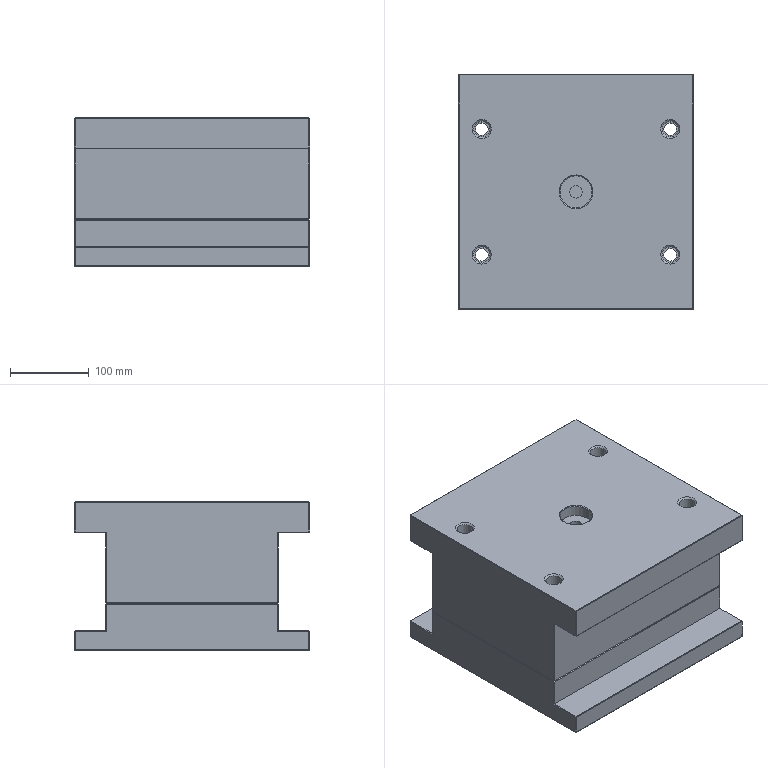NC program | NX | posted with a generic post | part box 300 x 300 x 190 mm
Lines 6041 to 6235 of 6235:
(刀补 , TOOL : D10JING)
N12062 T09 M6
N12064 G54
N12066 G17 G0 G90 X-120. Y80. S3500 M3
N12068 G43 Z30. H9
N12070 Z0.5
N12072 G41 G94 G1 X-120.011 Y79.901 F1200. D9
N12074 G3 X-117.05 Y80. R1.482
N12076 X-117.05 Y80. Z-2. I-2.95 J0.
N12078 X-117.05 Y80. Z-4.5 I-2.95 J0.
N12080 X-117.05 Y80. Z-7. I-2.95 J0.
N12082 X-117.05 Y80. Z-9.5 I-2.95 J0.
N12084 X-117.05 Y80. Z-12. I-2.95 J0.
N12086 X-117.05 Y80. Z-14.5 I-2.95 J0.
N12088 X-117.05 Y80. Z-17. I-2.95 J0.
N12090 X-117.05 Y80. Z-19.5 I-2.95 J0.
N12092 X-117.05 Y80. Z-22. I-2.95 J0.
N12094 X-117.05 Y80. Z-24.5 I-2.95 J0.
N12096 X-117.05 Y80. Z-27. I-2.95 J0.
N12098 X-117.05 Y80. Z-29.5 I-2.95 J0.
N12100 X-117.05 Y80. Z-32. I-2.95 J0.
N12102 X-117.05 Y80. Z-34.5 I-2.95 J0.
N12104 X-117.05 Y80. Z-37. I-2.95 J0.
N12106 X-117.05 Y80. Z-39.5 I-2.95 J0.
N12108 X-117.05 Y80. Z-42. I-2.95 J0.
N12110 X-117.05 Y80. Z-44.5 I-2.95 J0.
N12112 X-117.05 Y80. Z-47. I-2.95 J0.
N12114 X-117.05 Y80. Z-49.5 I-2.95 J0.
N12116 X-117.05 Y80. Z-52. I-2.95 J0.
N12118 X-117.05 Y80. Z-54.5 I-2.95 J0.
N12120 X-117.05 Y80. Z-57. I-2.95 J0.
N12122 X-117.05 Y80. Z-59.5 I-2.95 J0.
N12124 X-119.088 Y82.806 Z-60. R2.95
N12126 X-122.806 Y80.912 R2.95
N12128 X-119.088 Y82.806 R-2.95
N12130 X-120.098 Y80.021 R1.482
N12132 G40
N12134 G1 X-120. Y80.
N12136 G0 Z30.
N12138 Y-80.
N12140 Z0.5
N12142 G41 G1 X-120.011 Y-80.099
N12144 G3 X-117.05 Y-80. R1.482
N12146 X-117.05 Y-80. Z-2. I-2.95 J0.
N12148 X-117.05 Y-80. Z-4.5 I-2.95 J0.
N12150 X-117.05 Y-80. Z-7. I-2.95 J0.
N12152 X-117.05 Y-80. Z-9.5 I-2.95 J0.
N12154 X-117.05 Y-80. Z-12. I-2.95 J0.
N12156 X-117.05 Y-80. Z-14.5 I-2.95 J0.
N12158 X-117.05 Y-80. Z-17. I-2.95 J0.
N12160 X-117.05 Y-80. Z-19.5 I-2.95 J0.
N12162 X-117.05 Y-80. Z-22. I-2.95 J0.
N12164 X-117.05 Y-80. Z-24.5 I-2.95 J0.
N12166 X-117.05 Y-80. Z-27. I-2.95 J0.
N12168 X-117.05 Y-80. Z-29.5 I-2.95 J0.
N12170 X-117.05 Y-80. Z-32. I-2.95 J0.
N12172 X-117.05 Y-80. Z-34.5 I-2.95 J0.
N12174 X-117.05 Y-80. Z-37. I-2.95 J0.
N12176 X-117.05 Y-80. Z-39.5 I-2.95 J0.
N12178 X-117.05 Y-80. Z-42. I-2.95 J0.
N12180 X-117.05 Y-80. Z-44.5 I-2.95 J0.
N12182 X-117.05 Y-80. Z-47. I-2.95 J0.
N12184 X-117.05 Y-80. Z-49.5 I-2.95 J0.
N12186 X-117.05 Y-80. Z-52. I-2.95 J0.
N12188 X-117.05 Y-80. Z-54.5 I-2.95 J0.
N12190 X-117.05 Y-80. Z-57. I-2.95 J0.
N12192 X-117.05 Y-80. Z-59.5 I-2.95 J0.
N12194 X-119.088 Y-77.194 Z-60. R2.95
N12196 X-122.806 Y-79.088 R2.95
N12198 X-119.088 Y-77.194 R-2.95
N12200 X-120.098 Y-79.979 R1.482
N12202 G40
N12204 G1 X-120. Y-80.
N12206 G0 Z30.
N12208 X120.
N12210 Z0.5
N12212 G41 G1 X119.989 Y-80.099
N12214 G3 X122.95 Y-80. R1.482
N12216 X122.95 Y-80. Z-2. I-2.95 J0.
N12218 X122.95 Y-80. Z-4.5 I-2.95 J0.
N12220 X122.95 Y-80. Z-7. I-2.95 J0.
N12222 X122.95 Y-80. Z-9.5 I-2.95 J0.
N12224 X122.95 Y-80. Z-12. I-2.95 J0.
N12226 X122.95 Y-80. Z-14.5 I-2.95 J0.
N12228 X122.95 Y-80. Z-17. I-2.95 J0.
N12230 X122.95 Y-80. Z-19.5 I-2.95 J0.
N12232 X122.95 Y-80. Z-22. I-2.95 J0.
N12234 X122.95 Y-80. Z-24.5 I-2.95 J0.
N12236 X122.95 Y-80. Z-27. I-2.95 J0.
N12238 X122.95 Y-80. Z-29.5 I-2.95 J0.
N12240 X122.95 Y-80. Z-32. I-2.95 J0.
N12242 X122.95 Y-80. Z-34.5 I-2.95 J0.
N12244 X122.95 Y-80. Z-37. I-2.95 J0.
N12246 X122.95 Y-80. Z-39.5 I-2.95 J0.
N12248 X122.95 Y-80. Z-42. I-2.95 J0.
N12250 X122.95 Y-80. Z-44.5 I-2.95 J0.
N12252 X122.95 Y-80. Z-47. I-2.95 J0.
N12254 X122.95 Y-80. Z-49.5 I-2.95 J0.
N12256 X122.95 Y-80. Z-52. I-2.95 J0.
N12258 X122.95 Y-80. Z-54.5 I-2.95 J0.
N12260 X122.95 Y-80. Z-57. I-2.95 J0.
N12262 X122.95 Y-80. Z-59.5 I-2.95 J0.
N12264 X120.912 Y-77.194 Z-60. R2.95
N12266 X117.194 Y-79.088 R2.95
N12268 X120.912 Y-77.194 R-2.95
N12270 X119.902 Y-79.979 R1.482
N12272 G40
N12274 G1 X120. Y-80.
N12276 G0 Z30.
N12278 Y80.
N12280 Z0.5
N12282 G41 G1 X119.989 Y79.901
N12284 G3 X122.95 Y80. R1.482
N12286 X122.95 Y80. Z-2. I-2.95 J0.
N12288 X122.95 Y80. Z-4.5 I-2.95 J0.
N12290 X122.95 Y80. Z-7. I-2.95 J0.
N12292 X122.95 Y80. Z-9.5 I-2.95 J0.
N12294 X122.95 Y80. Z-12. I-2.95 J0.
N12296 X122.95 Y80. Z-14.5 I-2.95 J0.
N12298 X122.95 Y80. Z-17. I-2.95 J0.
N12300 X122.95 Y80. Z-19.5 I-2.95 J0.
N12302 X122.95 Y80. Z-22. I-2.95 J0.
N12304 X122.95 Y80. Z-24.5 I-2.95 J0.
N12306 X122.95 Y80. Z-27. I-2.95 J0.
N12308 X122.95 Y80. Z-29.5 I-2.95 J0.
N12310 X122.95 Y80. Z-32. I-2.95 J0.
N12312 X122.95 Y80. Z-34.5 I-2.95 J0.
N12314 X122.95 Y80. Z-37. I-2.95 J0.
N12316 X122.95 Y80. Z-39.5 I-2.95 J0.
N12318 X122.95 Y80. Z-42. I-2.95 J0.
N12320 X122.95 Y80. Z-44.5 I-2.95 J0.
N12322 X122.95 Y80. Z-47. I-2.95 J0.
N12324 X122.95 Y80. Z-49.5 I-2.95 J0.
N12326 X122.95 Y80. Z-52. I-2.95 J0.
N12328 X122.95 Y80. Z-54.5 I-2.95 J0.
N12330 X122.95 Y80. Z-57. I-2.95 J0.
N12332 X122.95 Y80. Z-59.5 I-2.95 J0.
N12334 X120.912 Y82.806 Z-60. R2.95
N12336 X117.194 Y80.912 R2.95
N12338 X120.912 Y82.806 R-2.95
N12340 X119.902 Y80.021 R1.482
N12342 G40
N12344 G1 X120. Y80.
N12346 G0 Z30.
(刀补2 , TOOL : D10JING)
N12348 X43.391 Y-1.492 S4000
N12350 Z0.493
N12352 G1 Z-1.007
N12354 G41 X43.485 Y-1.457
N12356 X44.509 Y-0.866
N12358 G3 X45.009 Y0. R1.
N12360 X0. Y45.009 R45.009
N12362 X45.009 Y0. R-45.009
N12364 X44.509 Y0.866 R1.
N12366 G1 X43.485 Y1.457
N12368 G40
N12370 X43.391 Y1.492
N12372 Z0.493
N12374 G0 Z30.
N12376 X1.478 Y22.418
N12378 Z-32.822
N12380 G1 Z-34.322
N12382 G41 X1.443 Y22.512
N12384 X0.866 Y23.512
N12386 G3 X0. Y24.012 R1.
N12388 G1 X-19.584
N12390 G3 X-29.758 Y18.329 R11.95
N12392 X29.758 Y18.329 R-34.95
N12394 X19.584 Y24.012 R11.95
N12396 G1 X0.
N12398 G3 X-0.866 Y23.512 R1.
N12400 G1 X-1.443 Y22.512
N12402 G40
N12404 X-1.478 Y22.418
N12406 Z-32.822
N12408 G0 Z30.
N12410 X18.284 Y27.9
N12412 Z-27.822
N12414 G1 Z-29.322
N12416 G41 X18.303 Y27.998
N12418 X18.317 Y29.19
N12420 G3 X17.827 Y30.062 R1.
N12422 X-17.827 Y30.062 R34.95
N12424 X-18.317 Y29.19 R1.
N12426 G1 X-18.303 Y27.998
N12428 G40
N12430 X-18.284 Y27.9
N12432 Z-27.822
N12434 G0 Z30.
N12436 M5
N12438 M2